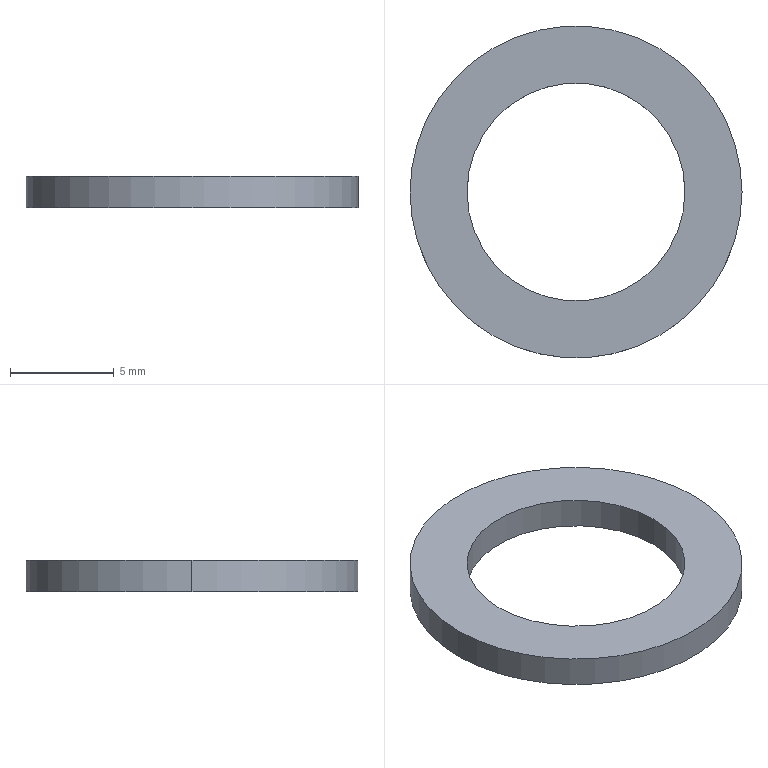Part | SolidWorks | features Extrusion 1 | 1 solid | 6 faces | box 16 x 16 x 1.5 mm | volume 171.708 mm3 | cylinder 4 | plane 2 | commonest cylinder face diameters 10.5 x2 16 x2
STEP:
#1=CARTESIAN_POINT('',(-5.25,0.,1.5));
#2=VERTEX_POINT('',#1);
#3=CARTESIAN_POINT('',(5.25,0.,1.5));
#4=VERTEX_POINT('',#3);
#5=CARTESIAN_POINT('',(0.,0.,1.5));
#6=DIRECTION('',(0.,0.,1.));
#7=DIRECTION('',(1.,0.,0.));
#8=AXIS2_PLACEMENT_3D('',#5,#6,#7);
#9=CIRCLE('',#8,5.25);
#10=EDGE_CURVE('',#2,#4,#9,.T.);
#11=ORIENTED_EDGE('',*,*,#10,.T.);
#12=CARTESIAN_POINT('',(5.25,0.,0.));
#13=VERTEX_POINT('',#12);
#14=CARTESIAN_POINT('',(5.25,0.,1.5));
#15=DIRECTION('',(0.,0.,-1.));
#16=VECTOR('',#15,1000.);
#17=LINE('',#14,#16);
#18=EDGE_CURVE('',#4,#13,#17,.T.);
#19=ORIENTED_EDGE('',*,*,#18,.T.);
#20=CARTESIAN_POINT('',(-5.25,0.,0.));
#21=VERTEX_POINT('',#20);
#22=CARTESIAN_POINT('',(0.,0.,0.));
#23=DIRECTION('',(0.,0.,1.));
#24=DIRECTION('',(1.,0.,0.));
#25=AXIS2_PLACEMENT_3D('',#22,#23,#24);
#26=CIRCLE('',#25,5.25);
#27=EDGE_CURVE('',#21,#13,#26,.T.);
#28=ORIENTED_EDGE('',*,*,#27,.F.);
#29=CARTESIAN_POINT('',(-5.25,0.,1.5));
#30=DIRECTION('',(0.,0.,-1.));
#31=VECTOR('',#30,1000.);
#32=LINE('',#29,#31);
#33=EDGE_CURVE('',#2,#21,#32,.T.);
#34=ORIENTED_EDGE('',*,*,#33,.F.);
#35=EDGE_LOOP('',(#11,#19,#28,#34));
#36=FACE_OUTER_BOUND('',#35,.T.);
#37=CARTESIAN_POINT('',(0.,0.,1.5));
#38=DIRECTION('',(0.,0.,-1.));
#39=DIRECTION('',(-1.,0.,0.));
#40=AXIS2_PLACEMENT_3D('',#37,#38,#39);
#41=CYLINDRICAL_SURFACE('',#40,5.25);
#42=ADVANCED_FACE('',(#36),#41,.F.);
#43=CARTESIAN_POINT('',(8.,0.,1.5));
#44=VERTEX_POINT('',#43);
#45=CARTESIAN_POINT('',(-8.,0.,1.5));
#46=VERTEX_POINT('',#45);
#47=CARTESIAN_POINT('',(0.,0.,1.5));
#48=DIRECTION('',(0.,0.,1.));
#49=DIRECTION('',(1.,0.,0.));
#50=AXIS2_PLACEMENT_3D('',#47,#48,#49);
#51=CIRCLE('',#50,8.);
#52=EDGE_CURVE('',#44,#46,#51,.T.);
#53=ORIENTED_EDGE('',*,*,#52,.F.);
#54=CARTESIAN_POINT('',(8.,0.,0.));
#55=VERTEX_POINT('',#54);
#56=CARTESIAN_POINT('',(8.,0.,1.5));
#57=DIRECTION('',(0.,0.,-1.));
#58=VECTOR('',#57,1000.);
#59=LINE('',#56,#58);
#60=EDGE_CURVE('',#44,#55,#59,.T.);
#61=ORIENTED_EDGE('',*,*,#60,.T.);
#62=CARTESIAN_POINT('',(-8.,0.,0.));
#63=VERTEX_POINT('',#62);
#64=CARTESIAN_POINT('',(0.,0.,0.));
#65=DIRECTION('',(0.,0.,1.));
#66=DIRECTION('',(1.,0.,0.));
#67=AXIS2_PLACEMENT_3D('',#64,#65,#66);
#68=CIRCLE('',#67,8.);
#69=EDGE_CURVE('',#55,#63,#68,.T.);
#70=ORIENTED_EDGE('',*,*,#69,.T.);
#71=CARTESIAN_POINT('',(-8.,0.,1.5));
#72=DIRECTION('',(0.,0.,-1.));
#73=VECTOR('',#72,1000.);
#74=LINE('',#71,#73);
#75=EDGE_CURVE('',#46,#63,#74,.T.);
#76=ORIENTED_EDGE('',*,*,#75,.F.);
#77=EDGE_LOOP('',(#53,#61,#70,#76));
#78=FACE_OUTER_BOUND('',#77,.T.);
#79=CARTESIAN_POINT('',(0.,0.,1.5));
#80=DIRECTION('',(0.,0.,-1.));
#81=DIRECTION('',(-1.,0.,0.));
#82=AXIS2_PLACEMENT_3D('',#79,#80,#81);
#83=CYLINDRICAL_SURFACE('',#82,8.);
#84=ADVANCED_FACE('',(#78),#83,.T.);
#85=CARTESIAN_POINT('',(0.,0.,1.5));
#86=DIRECTION('',(0.,0.,1.));
#87=DIRECTION('',(1.,0.,0.));
#88=AXIS2_PLACEMENT_3D('',#85,#86,#87);
#89=CIRCLE('',#88,8.);
#90=EDGE_CURVE('',#46,#44,#89,.T.);
#91=ORIENTED_EDGE('',*,*,#90,.T.);
#92=ORIENTED_EDGE('',*,*,#52,.T.);
#93=EDGE_LOOP('',(#91,#92));
#94=FACE_OUTER_BOUND('',#93,.T.);
#95=ORIENTED_EDGE('',*,*,#10,.F.);
#96=CARTESIAN_POINT('',(0.,0.,1.5));
#97=DIRECTION('',(0.,0.,1.));
#98=DIRECTION('',(1.,0.,0.));
#99=AXIS2_PLACEMENT_3D('',#96,#97,#98);
#100=CIRCLE('',#99,5.25);
#101=EDGE_CURVE('',#4,#2,#100,.T.);
#102=ORIENTED_EDGE('',*,*,#101,.F.);
#103=EDGE_LOOP('',(#95,#102));
#104=FACE_BOUND('',#103,.T.);
#105=CARTESIAN_POINT('',(0.,0.,1.5));
#106=DIRECTION('',(0.,0.,1.));
#107=DIRECTION('',(1.,0.,0.));
#108=AXIS2_PLACEMENT_3D('',#105,#106,#107);
#109=PLANE('',#108);
#110=ADVANCED_FACE('',(#94,#104),#109,.T.);
#111=CARTESIAN_POINT('',(0.,0.,0.));
#112=DIRECTION('',(0.,0.,1.));
#113=DIRECTION('',(1.,0.,0.));
#114=AXIS2_PLACEMENT_3D('',#111,#112,#113);
#115=CIRCLE('',#114,8.);
#116=EDGE_CURVE('',#63,#55,#115,.T.);
#117=ORIENTED_EDGE('',*,*,#116,.F.);
#118=ORIENTED_EDGE('',*,*,#69,.F.);
#119=EDGE_LOOP('',(#117,#118));
#120=FACE_OUTER_BOUND('',#119,.T.);
#121=ORIENTED_EDGE('',*,*,#27,.T.);
#122=CARTESIAN_POINT('',(0.,0.,0.));
#123=DIRECTION('',(0.,0.,1.));
#124=DIRECTION('',(1.,0.,0.));
#125=AXIS2_PLACEMENT_3D('',#122,#123,#124);
#126=CIRCLE('',#125,5.25);
#127=EDGE_CURVE('',#13,#21,#126,.T.);
#128=ORIENTED_EDGE('',*,*,#127,.T.);
#129=EDGE_LOOP('',(#121,#128));
#130=FACE_BOUND('',#129,.T.);
#131=CARTESIAN_POINT('',(0.,0.,0.));
#132=DIRECTION('',(0.,0.,1.));
#133=DIRECTION('',(1.,0.,0.));
#134=AXIS2_PLACEMENT_3D('',#131,#132,#133);
#135=PLANE('',#134);
#136=ADVANCED_FACE('',(#120,#130),#135,.F.);
#137=ORIENTED_EDGE('',*,*,#60,.F.);
#138=ORIENTED_EDGE('',*,*,#90,.F.);
#139=ORIENTED_EDGE('',*,*,#75,.T.);
#140=ORIENTED_EDGE('',*,*,#116,.T.);
#141=EDGE_LOOP('',(#137,#138,#139,#140));
#142=FACE_OUTER_BOUND('',#141,.T.);
#143=CARTESIAN_POINT('',(0.,0.,1.5));
#144=DIRECTION('',(0.,0.,-1.));
#145=DIRECTION('',(-1.,0.,0.));
#146=AXIS2_PLACEMENT_3D('',#143,#144,#145);
#147=CYLINDRICAL_SURFACE('',#146,8.);
#148=ADVANCED_FACE('',(#142),#147,.T.);
#149=ORIENTED_EDGE('',*,*,#18,.F.);
#150=ORIENTED_EDGE('',*,*,#101,.T.);
#151=ORIENTED_EDGE('',*,*,#33,.T.);
#152=ORIENTED_EDGE('',*,*,#127,.F.);
#153=EDGE_LOOP('',(#149,#150,#151,#152));
#154=FACE_OUTER_BOUND('',#153,.T.);
#155=CARTESIAN_POINT('',(0.,0.,1.5));
#156=DIRECTION('',(0.,0.,-1.));
#157=DIRECTION('',(-1.,0.,0.));
#158=AXIS2_PLACEMENT_3D('',#155,#156,#157);
#159=CYLINDRICAL_SURFACE('',#158,5.25);
#160=ADVANCED_FACE('',(#154),#159,.F.);
#161=CLOSED_SHELL('',(#42,#84,#110,#136,#148,#160));
#162=MANIFOLD_SOLID_BREP('',#161);
#163=CARTESIAN_POINT('',(0.,0.,0.));
#164=DIRECTION('',(0.,0.,1.));
#165=DIRECTION('',(1.,0.,0.));
#166=AXIS2_PLACEMENT_3D('',#163,#164,#165);
#167=(LENGTH_UNIT()NAMED_UNIT(*)SI_UNIT(.MILLI.,.METRE.));
#168=UNCERTAINTY_MEASURE_WITH_UNIT(LENGTH_MEASURE(0.00001),#167,'','');
#169=(NAMED_UNIT(*)PLANE_ANGLE_UNIT()SI_UNIT($,.RADIAN.));
#170=(NAMED_UNIT(*)SI_UNIT($,.STERADIAN.)SOLID_ANGLE_UNIT());
#171=(GEOMETRIC_REPRESENTATION_CONTEXT(3)GLOBAL_UNCERTAINTY_ASSIGNED_CONTEXT((#168))GLOBAL_UNIT_ASSIGNED_CONTEXT((#167,#169,#170))REPRESENTATION_CONTEXT('',''));
#172=ADVANCED_BREP_SHAPE_REPRESENTATION('',(#162,#166),#171);